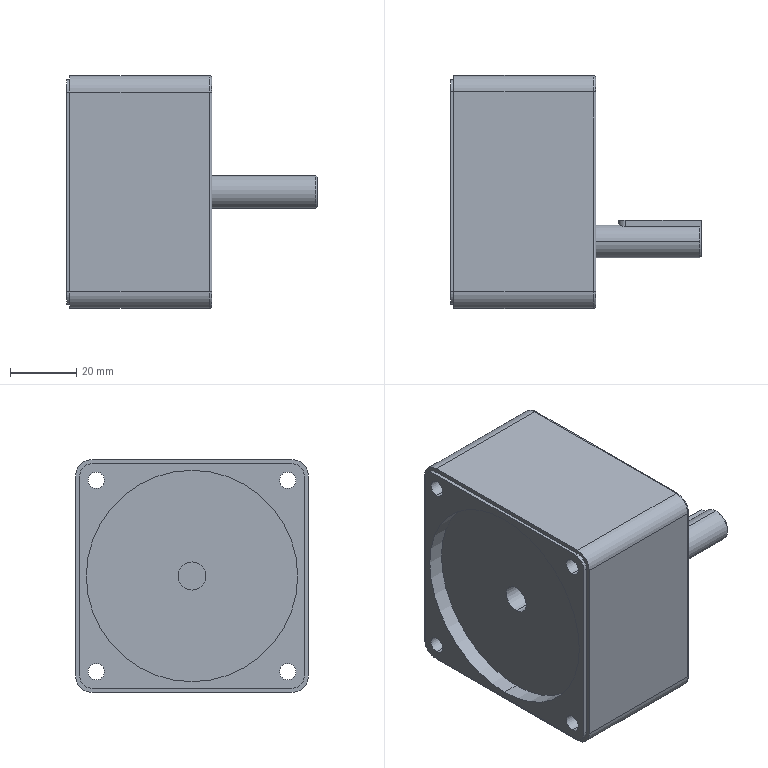Part | STEP file | QA-15YT01-25-2 | 2 solids | 194 faces | box 76 x 70.5 x 70.5 mm | volume 194650 mm3 | spline 80 | plane 66 | cylinder 37 | cone 11 | commonest cylinder face diameters 5 x8 10 x6 1.5 x4 7.5 x4 64 x4 3.15 x2